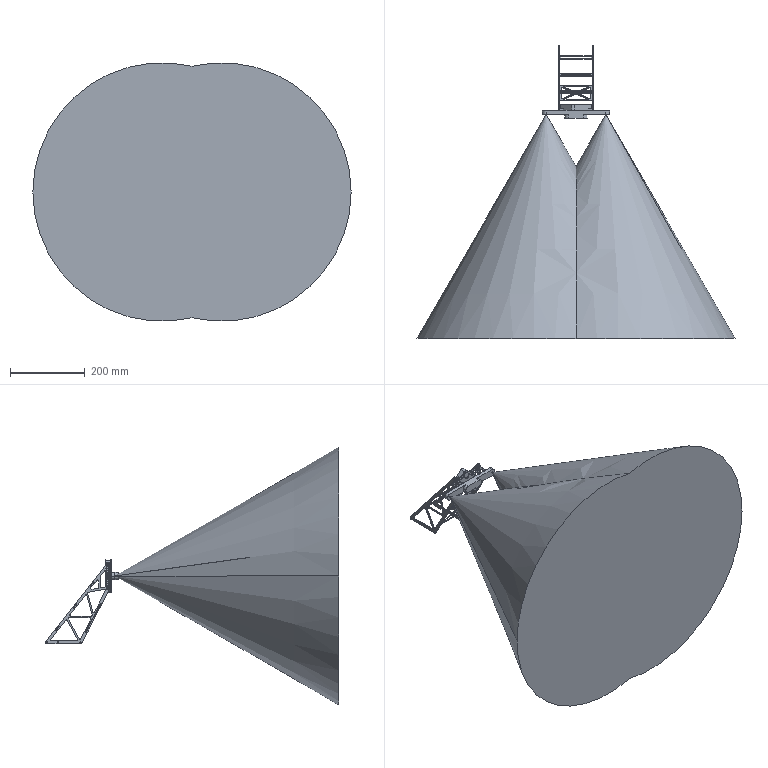Part | SolidWorks | 16 solids | 786 faces | box 852.82 x 786 x 692.82 mm | volume 107026744 mm3 | cylinder 453 | plane 321 | cone 12 | commonest cylinder face diameters 2 x78 3.1 x76 3 x69 1.2 x44 5 x42 1.05 x36